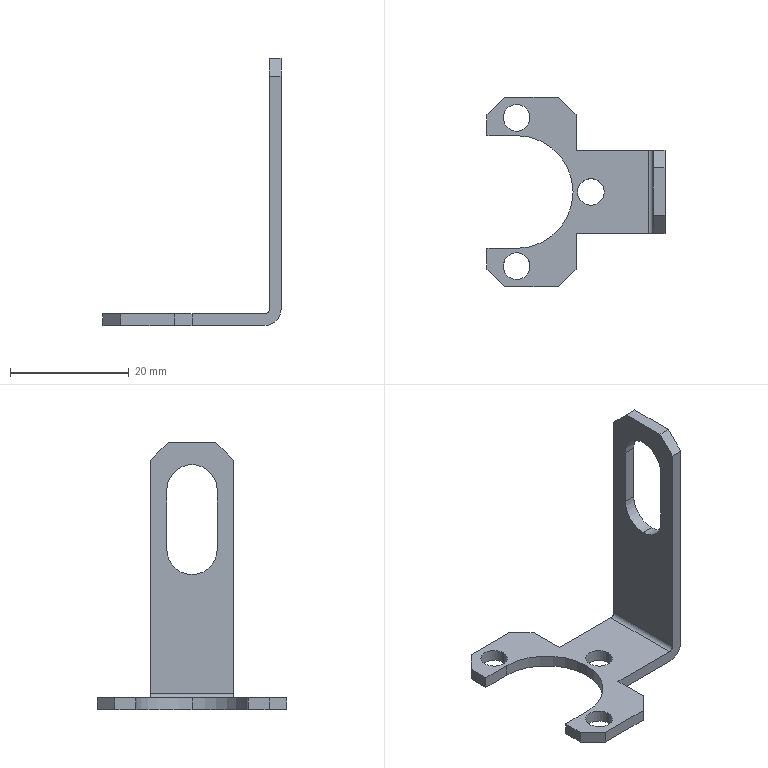Part | STEP file | Proximity mounting bent plate | 1 solid | 36 faces | box 30 x 32 x 45 mm | volume 1657 mm3 | plane 23 | cylinder 13 | commonest cylinder face diameters 4.5 x6 8.5 x3 19 x2 1.473 x1 5.473 x1